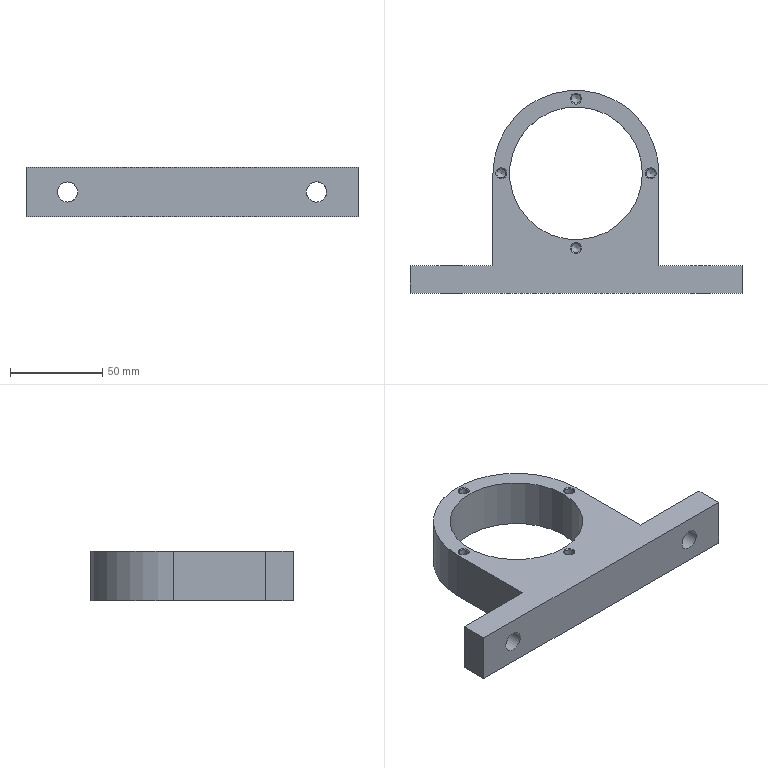Part | NX | features DATUM_CSYS 9, SKETCH 8, EXTRACT_FACE 4, HOLE PACKAGE 4, SIMPLE HOLE 4, SYMBOLIC_THREAD 4, EXTRUDE 3, Instance Feature 3, Pattern Feature 1 | 1 solid | 31 faces | box 180 x 110 x 27 mm | volume 165663 mm3 | plane 12 | cylinder 11 | cone 8 | commonest cylinder face diameters 5 x4 6 x3 11 x2 72 x1 90 x1
STEP:
#1=CARTESIAN_POINT('',(-67.5,-65.,8.));
#2=VERTEX_POINT('',#1);
#3=CARTESIAN_POINT('',(-67.5,-65.,13.5));
#4=DIRECTION('',(0.,-1.,0.));
#5=DIRECTION('',(0.,0.,-1.));
#6=AXIS2_PLACEMENT_3D('',#3,#4,#5);
#7=CIRCLE('',#6,5.5);
#8=EDGE_CURVE('',#2,#2,#7,.F.);
#9=ORIENTED_EDGE('',*,*,#8,.T.);
#10=EDGE_LOOP('',(#9));
#11=FACE_BOUND('',#10,.T.);
#12=CARTESIAN_POINT('',(67.5,-65.,8.));
#13=VERTEX_POINT('',#12);
#14=CARTESIAN_POINT('',(67.5,-65.,13.5));
#15=DIRECTION('',(0.,-1.,0.));
#16=DIRECTION('',(0.,0.,-1.));
#17=AXIS2_PLACEMENT_3D('',#14,#15,#16);
#18=CIRCLE('',#17,5.5);
#19=EDGE_CURVE('',#13,#13,#18,.T.);
#20=ORIENTED_EDGE('',*,*,#19,.F.);
#21=EDGE_LOOP('',(#20));
#22=FACE_BOUND('',#21,.T.);
#23=CARTESIAN_POINT('',(90.,-65.,0.));
#24=VERTEX_POINT('',#23);
#25=CARTESIAN_POINT('',(-90.,-65.,0.));
#26=VERTEX_POINT('',#25);
#27=CARTESIAN_POINT('',(90.,-65.,0.));
#28=DIRECTION('',(-1.,0.,0.));
#29=VECTOR('',#28,1000.);
#30=LINE('',#27,#29);
#31=EDGE_CURVE('',#24,#26,#30,.T.);
#32=ORIENTED_EDGE('',*,*,#31,.F.);
#33=CARTESIAN_POINT('',(90.,-65.,27.));
#34=VERTEX_POINT('',#33);
#35=CARTESIAN_POINT('',(90.,-65.,27.));
#36=DIRECTION('',(0.,0.,-1.));
#37=VECTOR('',#36,1000.);
#38=LINE('',#35,#37);
#39=EDGE_CURVE('',#34,#24,#38,.T.);
#40=ORIENTED_EDGE('',*,*,#39,.F.);
#41=CARTESIAN_POINT('',(-90.,-65.,27.));
#42=VERTEX_POINT('',#41);
#43=CARTESIAN_POINT('',(90.,-65.,27.));
#44=DIRECTION('',(-1.,0.,0.));
#45=VECTOR('',#44,1000.);
#46=LINE('',#43,#45);
#47=EDGE_CURVE('',#34,#42,#46,.T.);
#48=ORIENTED_EDGE('',*,*,#47,.T.);
#49=CARTESIAN_POINT('',(-90.,-65.,27.));
#50=DIRECTION('',(0.,0.,-1.));
#51=VECTOR('',#50,1000.);
#52=LINE('',#49,#51);
#53=EDGE_CURVE('',#42,#26,#52,.T.);
#54=ORIENTED_EDGE('',*,*,#53,.T.);
#55=EDGE_LOOP('',(#32,#40,#48,#54));
#56=FACE_BOUND('',#55,.T.);
#57=CARTESIAN_POINT('',(90.,-65.,27.));
#58=DIRECTION('',(0.,-1.,0.));
#59=DIRECTION('',(0.,0.,-1.));
#60=AXIS2_PLACEMENT_3D('',#57,#58,#59);
#61=PLANE('',#60);
#62=ADVANCED_FACE('',(#11,#22,#56),#61,.T.);
#63=CARTESIAN_POINT('',(-90.,-50.,0.));
#64=VERTEX_POINT('',#63);
#65=CARTESIAN_POINT('',(-90.,-65.,0.));
#66=DIRECTION('',(0.,1.,0.));
#67=VECTOR('',#66,1000.);
#68=LINE('',#65,#67);
#69=EDGE_CURVE('',#26,#64,#68,.T.);
#70=ORIENTED_EDGE('',*,*,#69,.F.);
#71=ORIENTED_EDGE('',*,*,#53,.F.);
#72=CARTESIAN_POINT('',(-90.,-50.,27.));
#73=VERTEX_POINT('',#72);
#74=CARTESIAN_POINT('',(-90.,-65.,27.));
#75=DIRECTION('',(0.,1.,0.));
#76=VECTOR('',#75,1000.);
#77=LINE('',#74,#76);
#78=EDGE_CURVE('',#42,#73,#77,.T.);
#79=ORIENTED_EDGE('',*,*,#78,.T.);
#80=CARTESIAN_POINT('',(-90.,-50.,27.));
#81=DIRECTION('',(0.,0.,-1.));
#82=VECTOR('',#81,1000.);
#83=LINE('',#80,#82);
#84=EDGE_CURVE('',#73,#64,#83,.T.);
#85=ORIENTED_EDGE('',*,*,#84,.T.);
#86=EDGE_LOOP('',(#70,#71,#79,#85));
#87=FACE_BOUND('',#86,.T.);
#88=CARTESIAN_POINT('',(-90.,-65.,27.));
#89=DIRECTION('',(-1.,0.,0.));
#90=DIRECTION('',(0.,-1.,0.));
#91=AXIS2_PLACEMENT_3D('',#88,#89,#90);
#92=PLANE('',#91);
#93=ADVANCED_FACE('',(#87),#92,.T.);
#94=CARTESIAN_POINT('',(-62.,-50.,13.5));
#95=VERTEX_POINT('',#94);
#96=CARTESIAN_POINT('',(-67.5,-50.,13.5));
#97=DIRECTION('',(0.,-1.,0.));
#98=DIRECTION('',(1.,0.,0.));
#99=AXIS2_PLACEMENT_3D('',#96,#97,#98);
#100=CIRCLE('',#99,5.5);
#101=EDGE_CURVE('',#95,#95,#100,.T.);
#102=ORIENTED_EDGE('',*,*,#101,.T.);
#103=EDGE_LOOP('',(#102));
#104=FACE_BOUND('',#103,.T.);
#105=CARTESIAN_POINT('',(-45.,-50.,0.));
#106=VERTEX_POINT('',#105);
#107=CARTESIAN_POINT('',(-90.,-50.,0.));
#108=DIRECTION('',(1.,0.,0.));
#109=VECTOR('',#108,1000.);
#110=LINE('',#107,#109);
#111=EDGE_CURVE('',#64,#106,#110,.T.);
#112=ORIENTED_EDGE('',*,*,#111,.F.);
#113=ORIENTED_EDGE('',*,*,#84,.F.);
#114=CARTESIAN_POINT('',(-45.,-50.,27.));
#115=VERTEX_POINT('',#114);
#116=CARTESIAN_POINT('',(-90.,-50.,27.));
#117=DIRECTION('',(1.,0.,0.));
#118=VECTOR('',#117,1000.);
#119=LINE('',#116,#118);
#120=EDGE_CURVE('',#73,#115,#119,.T.);
#121=ORIENTED_EDGE('',*,*,#120,.T.);
#122=CARTESIAN_POINT('',(-45.,-50.,27.));
#123=DIRECTION('',(0.,0.,-1.));
#124=VECTOR('',#123,1000.);
#125=LINE('',#122,#124);
#126=EDGE_CURVE('',#115,#106,#125,.T.);
#127=ORIENTED_EDGE('',*,*,#126,.T.);
#128=EDGE_LOOP('',(#112,#113,#121,#127));
#129=FACE_BOUND('',#128,.T.);
#130=CARTESIAN_POINT('',(-90.,-50.,27.));
#131=DIRECTION('',(0.,1.,0.));
#132=DIRECTION('',(0.,0.,1.));
#133=AXIS2_PLACEMENT_3D('',#130,#131,#132);
#134=PLANE('',#133);
#135=ADVANCED_FACE('',(#104,#129),#134,.T.);
#136=CARTESIAN_POINT('',(-45.,0.,0.));
#137=VERTEX_POINT('',#136);
#138=CARTESIAN_POINT('',(-45.,-50.,0.));
#139=DIRECTION('',(0.,1.,0.));
#140=VECTOR('',#139,1000.);
#141=LINE('',#138,#140);
#142=EDGE_CURVE('',#106,#137,#141,.T.);
#143=ORIENTED_EDGE('',*,*,#142,.F.);
#144=ORIENTED_EDGE('',*,*,#126,.F.);
#145=CARTESIAN_POINT('',(-45.,0.,27.));
#146=VERTEX_POINT('',#145);
#147=CARTESIAN_POINT('',(-45.,-50.,27.));
#148=DIRECTION('',(0.,1.,0.));
#149=VECTOR('',#148,1000.);
#150=LINE('',#147,#149);
#151=EDGE_CURVE('',#115,#146,#150,.T.);
#152=ORIENTED_EDGE('',*,*,#151,.T.);
#153=CARTESIAN_POINT('',(-45.,0.,27.));
#154=DIRECTION('',(0.,0.,-1.));
#155=VECTOR('',#154,1000.);
#156=LINE('',#153,#155);
#157=EDGE_CURVE('',#146,#137,#156,.T.);
#158=ORIENTED_EDGE('',*,*,#157,.T.);
#159=EDGE_LOOP('',(#143,#144,#152,#158));
#160=FACE_BOUND('',#159,.T.);
#161=CARTESIAN_POINT('',(-45.,-50.,27.));
#162=DIRECTION('',(-1.,0.,0.));
#163=DIRECTION('',(0.,-1.,0.));
#164=AXIS2_PLACEMENT_3D('',#161,#162,#163);
#165=PLANE('',#164);
#166=ADVANCED_FACE('',(#160),#165,.T.);
#167=CARTESIAN_POINT('',(45.,0.,0.));
#168=VERTEX_POINT('',#167);
#169=CARTESIAN_POINT('',(0.,0.,0.));
#170=DIRECTION('',(0.,0.,-1.));
#171=DIRECTION('',(1.,0.,0.));
#172=AXIS2_PLACEMENT_3D('',#169,#170,#171);
#173=CIRCLE('',#172,45.);
#174=EDGE_CURVE('',#137,#168,#173,.T.);
#175=ORIENTED_EDGE('',*,*,#174,.F.);
#176=ORIENTED_EDGE('',*,*,#157,.F.);
#177=CARTESIAN_POINT('',(45.,0.,27.));
#178=VERTEX_POINT('',#177);
#179=CARTESIAN_POINT('',(0.,0.,27.));
#180=DIRECTION('',(0.,0.,-1.));
#181=DIRECTION('',(1.,0.,0.));
#182=AXIS2_PLACEMENT_3D('',#179,#180,#181);
#183=CIRCLE('',#182,45.);
#184=EDGE_CURVE('',#146,#178,#183,.T.);
#185=ORIENTED_EDGE('',*,*,#184,.T.);
#186=CARTESIAN_POINT('',(45.,0.,27.));
#187=DIRECTION('',(0.,0.,-1.));
#188=VECTOR('',#187,1000.);
#189=LINE('',#186,#188);
#190=EDGE_CURVE('',#178,#168,#189,.T.);
#191=ORIENTED_EDGE('',*,*,#190,.T.);
#192=EDGE_LOOP('',(#175,#176,#185,#191));
#193=FACE_BOUND('',#192,.T.);
#194=CARTESIAN_POINT('',(0.,0.,27.));
#195=DIRECTION('',(0.,0.,-1.));
#196=DIRECTION('',(-1.,0.,0.));
#197=AXIS2_PLACEMENT_3D('',#194,#195,#196);
#198=CYLINDRICAL_SURFACE('',#197,45.);
#199=ADVANCED_FACE('',(#193),#198,.T.);
#200=CARTESIAN_POINT('',(45.,-50.,0.));
#201=VERTEX_POINT('',#200);
#202=CARTESIAN_POINT('',(45.,0.,0.));
#203=DIRECTION('',(0.,-1.,0.));
#204=VECTOR('',#203,1000.);
#205=LINE('',#202,#204);
#206=EDGE_CURVE('',#168,#201,#205,.T.);
#207=ORIENTED_EDGE('',*,*,#206,.F.);
#208=ORIENTED_EDGE('',*,*,#190,.F.);
#209=CARTESIAN_POINT('',(45.,-50.,27.));
#210=VERTEX_POINT('',#209);
#211=CARTESIAN_POINT('',(45.,0.,27.));
#212=DIRECTION('',(0.,-1.,0.));
#213=VECTOR('',#212,1000.);
#214=LINE('',#211,#213);
#215=EDGE_CURVE('',#178,#210,#214,.T.);
#216=ORIENTED_EDGE('',*,*,#215,.T.);
#217=CARTESIAN_POINT('',(45.,-50.,27.));
#218=DIRECTION('',(0.,0.,-1.));
#219=VECTOR('',#218,1000.);
#220=LINE('',#217,#219);
#221=EDGE_CURVE('',#210,#201,#220,.T.);
#222=ORIENTED_EDGE('',*,*,#221,.T.);
#223=EDGE_LOOP('',(#207,#208,#216,#222));
#224=FACE_BOUND('',#223,.T.);
#225=CARTESIAN_POINT('',(45.,0.,27.));
#226=DIRECTION('',(1.,0.,0.));
#227=DIRECTION('',(0.,1.,0.));
#228=AXIS2_PLACEMENT_3D('',#225,#226,#227);
#229=PLANE('',#228);
#230=ADVANCED_FACE('',(#224),#229,.T.);
#231=CARTESIAN_POINT('',(62.,-50.,13.5));
#232=VERTEX_POINT('',#231);
#233=CARTESIAN_POINT('',(67.5,-50.,13.5));
#234=DIRECTION('',(0.,1.,0.));
#235=DIRECTION('',(-1.,0.,0.));
#236=AXIS2_PLACEMENT_3D('',#233,#234,#235);
#237=CIRCLE('',#236,5.5);
#238=EDGE_CURVE('',#232,#232,#237,.T.);
#239=ORIENTED_EDGE('',*,*,#238,.F.);
#240=EDGE_LOOP('',(#239));
#241=FACE_BOUND('',#240,.T.);
#242=CARTESIAN_POINT('',(90.,-50.,0.));
#243=VERTEX_POINT('',#242);
#244=CARTESIAN_POINT('',(45.,-50.,0.));
#245=DIRECTION('',(1.,0.,0.));
#246=VECTOR('',#245,1000.);
#247=LINE('',#244,#246);
#248=EDGE_CURVE('',#201,#243,#247,.T.);
#249=ORIENTED_EDGE('',*,*,#248,.F.);
#250=ORIENTED_EDGE('',*,*,#221,.F.);
#251=CARTESIAN_POINT('',(90.,-50.,27.));
#252=VERTEX_POINT('',#251);
#253=CARTESIAN_POINT('',(45.,-50.,27.));
#254=DIRECTION('',(1.,0.,0.));
#255=VECTOR('',#254,1000.);
#256=LINE('',#253,#255);
#257=EDGE_CURVE('',#210,#252,#256,.T.);
#258=ORIENTED_EDGE('',*,*,#257,.T.);
#259=CARTESIAN_POINT('',(90.,-50.,27.));
#260=DIRECTION('',(0.,0.,-1.));
#261=VECTOR('',#260,1000.);
#262=LINE('',#259,#261);
#263=EDGE_CURVE('',#252,#243,#262,.T.);
#264=ORIENTED_EDGE('',*,*,#263,.T.);
#265=EDGE_LOOP('',(#249,#250,#258,#264));
#266=FACE_BOUND('',#265,.T.);
#267=CARTESIAN_POINT('',(45.,-50.,27.));
#268=DIRECTION('',(0.,1.,0.));
#269=DIRECTION('',(-1.,0.,0.));
#270=AXIS2_PLACEMENT_3D('',#267,#268,#269);
#271=PLANE('',#270);
#272=ADVANCED_FACE('',(#241,#266),#271,.T.);
#273=CARTESIAN_POINT('',(90.,-50.,0.));
#274=DIRECTION('',(0.,-1.,0.));
#275=VECTOR('',#274,1000.);
#276=LINE('',#273,#275);
#277=EDGE_CURVE('',#243,#24,#276,.T.);
#278=ORIENTED_EDGE('',*,*,#277,.F.);
#279=ORIENTED_EDGE('',*,*,#263,.F.);
#280=CARTESIAN_POINT('',(90.,-50.,27.));
#281=DIRECTION('',(0.,-1.,0.));
#282=VECTOR('',#281,1000.);
#283=LINE('',#280,#282);
#284=EDGE_CURVE('',#252,#34,#283,.T.);
#285=ORIENTED_EDGE('',*,*,#284,.T.);
#286=ORIENTED_EDGE('',*,*,#39,.T.);
#287=EDGE_LOOP('',(#278,#279,#285,#286));
#288=FACE_BOUND('',#287,.T.);
#289=CARTESIAN_POINT('',(90.,-50.,27.));
#290=DIRECTION('',(1.,0.,0.));
#291=DIRECTION('',(0.,1.,0.));
#292=AXIS2_PLACEMENT_3D('',#289,#290,#291);
#293=PLANE('',#292);
#294=ADVANCED_FACE('',(#288),#293,.T.);
#295=CARTESIAN_POINT('',(36.,0.,27.));
#296=VERTEX_POINT('',#295);
#297=CARTESIAN_POINT('',(0.,0.,27.));
#298=DIRECTION('',(0.,0.,-1.));
#299=DIRECTION('',(1.,0.,0.));
#300=AXIS2_PLACEMENT_3D('',#297,#298,#299);
#301=CIRCLE('',#300,36.);
#302=EDGE_CURVE('',#296,#296,#301,.T.);
#303=ORIENTED_EDGE('',*,*,#302,.F.);
#304=EDGE_LOOP('',(#303));
#305=FACE_BOUND('',#304,.T.);
#306=CARTESIAN_POINT('',(36.,0.,0.));
#307=VERTEX_POINT('',#306);
#308=CARTESIAN_POINT('',(0.,0.,0.));
#309=DIRECTION('',(0.,0.,-1.));
#310=DIRECTION('',(1.,0.,0.));
#311=AXIS2_PLACEMENT_3D('',#308,#309,#310);
#312=CIRCLE('',#311,36.);
#313=EDGE_CURVE('',#307,#307,#312,.T.);
#314=ORIENTED_EDGE('',*,*,#313,.T.);
#315=EDGE_LOOP('',(#314));
#316=FACE_BOUND('',#315,.T.);
#317=CARTESIAN_POINT('',(0.,0.,27.));
#318=DIRECTION('',(0.,0.,-1.));
#319=DIRECTION('',(-1.,0.,0.));
#320=AXIS2_PLACEMENT_3D('',#317,#318,#319);
#321=CYLINDRICAL_SURFACE('',#320,36.);
#322=ADVANCED_FACE('',(#305,#316),#321,.F.);
#323=CARTESIAN_POINT('',(-3.,40.5,27.));
#324=VERTEX_POINT('',#323);
#325=CARTESIAN_POINT('',(0.,40.5,27.));
#326=DIRECTION('',(0.,0.,-1.));
#327=DIRECTION('',(-1.,0.,0.));
#328=AXIS2_PLACEMENT_3D('',#325,#326,#327);
#329=CIRCLE('',#328,3.);
#330=EDGE_CURVE('',#324,#324,#329,.T.);
#331=ORIENTED_EDGE('',*,*,#330,.T.);
#332=EDGE_LOOP('',(#331));
#333=FACE_BOUND('',#332,.T.);
#334=CARTESIAN_POINT('',(-43.5,0.,27.));
#335=VERTEX_POINT('',#334);
#336=CARTESIAN_POINT('',(-40.5,0.,27.));
#337=DIRECTION('',(0.,0.,-1.));
#338=DIRECTION('',(-1.,0.,0.));
#339=AXIS2_PLACEMENT_3D('',#336,#337,#338);
#340=CIRCLE('',#339,3.);
#341=EDGE_CURVE('',#335,#335,#340,.T.);
#342=ORIENTED_EDGE('',*,*,#341,.T.);
#343=EDGE_LOOP('',(#342));
#344=FACE_BOUND('',#343,.T.);
#345=CARTESIAN_POINT('',(-3.,-40.5,27.));
#346=VERTEX_POINT('',#345);
#347=CARTESIAN_POINT('',(0.,-40.5,27.));
#348=DIRECTION('',(0.,0.,-1.));
#349=DIRECTION('',(-1.,0.,0.));
#350=AXIS2_PLACEMENT_3D('',#347,#348,#349);
#351=CIRCLE('',#350,3.);
#352=EDGE_CURVE('',#346,#346,#351,.T.);
#353=ORIENTED_EDGE('',*,*,#352,.T.);
#354=EDGE_LOOP('',(#353));
#355=FACE_BOUND('',#354,.T.);
#356=CARTESIAN_POINT('',(37.5,0.,27.));
#357=VERTEX_POINT('',#356);
#358=CARTESIAN_POINT('',(40.5,0.,27.));
#359=DIRECTION('',(0.,0.,-1.));
#360=DIRECTION('',(-1.,0.,0.));
#361=AXIS2_PLACEMENT_3D('',#358,#359,#360);
#362=CIRCLE('',#361,3.);
#363=EDGE_CURVE('',#357,#357,#362,.T.);
#364=ORIENTED_EDGE('',*,*,#363,.T.);
#365=EDGE_LOOP('',(#364));
#366=FACE_BOUND('',#365,.T.);
#367=ORIENTED_EDGE('',*,*,#47,.F.);
#368=ORIENTED_EDGE('',*,*,#284,.F.);
#369=ORIENTED_EDGE('',*,*,#257,.F.);
#370=ORIENTED_EDGE('',*,*,#215,.F.);
#371=ORIENTED_EDGE('',*,*,#184,.F.);
#372=ORIENTED_EDGE('',*,*,#151,.F.);
#373=ORIENTED_EDGE('',*,*,#120,.F.);
#374=ORIENTED_EDGE('',*,*,#78,.F.);
#375=EDGE_LOOP('',(#367,#368,#369,#370,#371,#372,#373,#374));
#376=FACE_BOUND('',#375,.T.);
#377=ORIENTED_EDGE('',*,*,#302,.T.);
#378=EDGE_LOOP('',(#377));
#379=FACE_BOUND('',#378,.T.);
#380=CARTESIAN_POINT('',(0.,0.,27.));
#381=DIRECTION('',(0.,0.,-1.));
#382=DIRECTION('',(-1.,0.,0.));
#383=AXIS2_PLACEMENT_3D('',#380,#381,#382);
#384=PLANE('',#383);
#385=ADVANCED_FACE('',(#333,#344,#355,#366,#376,#379),#384,.F.);
#386=CARTESIAN_POINT('',(35.708,-17.152,0.));
#387=VERTEX_POINT('',#386);
#388=CARTESIAN_POINT('',(34.208,-19.75,0.));
#389=DIRECTION('',(0.,0.,-1.));
#390=DIRECTION('',(0.5,0.866,0.));
#391=AXIS2_PLACEMENT_3D('',#388,#389,#390);
#392=CIRCLE('',#391,3.);
#393=EDGE_CURVE('',#387,#387,#392,.T.);
#394=ORIENTED_EDGE('',*,*,#393,.F.);
#395=EDGE_LOOP('',(#394));
#396=FACE_BOUND('',#395,.T.);
#397=CARTESIAN_POINT('',(-32.708,-22.348,0.));
#398=VERTEX_POINT('',#397);
#399=CARTESIAN_POINT('',(-34.208,-19.75,0.));
#400=DIRECTION('',(0.,0.,-1.));
#401=DIRECTION('',(0.5,-0.866,0.));
#402=AXIS2_PLACEMENT_3D('',#399,#400,#401);
#403=CIRCLE('',#402,3.);
#404=EDGE_CURVE('',#398,#398,#403,.T.);
#405=ORIENTED_EDGE('',*,*,#404,.F.);
#406=EDGE_LOOP('',(#405));
#407=FACE_BOUND('',#406,.T.);
#408=CARTESIAN_POINT('',(-3.,39.5,0.));
#409=VERTEX_POINT('',#408);
#410=CARTESIAN_POINT('',(0.,39.5,0.));
#411=DIRECTION('',(0.,0.,-1.));
#412=DIRECTION('',(-1.,0.,0.));
#413=AXIS2_PLACEMENT_3D('',#410,#411,#412);
#414=CIRCLE('',#413,3.);
#415=EDGE_CURVE('',#409,#409,#414,.T.);
#416=ORIENTED_EDGE('',*,*,#415,.F.);
#417=EDGE_LOOP('',(#416));
#418=FACE_BOUND('',#417,.T.);
#419=ORIENTED_EDGE('',*,*,#31,.T.);
#420=ORIENTED_EDGE('',*,*,#69,.T.);
#421=ORIENTED_EDGE('',*,*,#111,.T.);
#422=ORIENTED_EDGE('',*,*,#142,.T.);
#423=ORIENTED_EDGE('',*,*,#174,.T.);
#424=ORIENTED_EDGE('',*,*,#206,.T.);
#425=ORIENTED_EDGE('',*,*,#248,.T.);
#426=ORIENTED_EDGE('',*,*,#277,.T.);
#427=EDGE_LOOP('',(#419,#420,#421,#422,#423,#424,#425,#426));
#428=FACE_BOUND('',#427,.T.);
#429=ORIENTED_EDGE('',*,*,#313,.F.);
#430=EDGE_LOOP('',(#429));
#431=FACE_BOUND('',#430,.T.);
#432=CARTESIAN_POINT('',(0.,0.,0.));
#433=DIRECTION('',(0.,0.,-1.));
#434=DIRECTION('',(-1.,0.,0.));
#435=AXIS2_PLACEMENT_3D('',#432,#433,#434);
#436=PLANE('',#435);
#437=ADVANCED_FACE('',(#396,#407,#418,#428,#431),#436,.T.);
#438=ORIENTED_EDGE('',*,*,#19,.T.);
#439=EDGE_LOOP('',(#438));
#440=FACE_BOUND('',#439,.T.);
#441=ORIENTED_EDGE('',*,*,#238,.T.);
#442=EDGE_LOOP('',(#441));
#443=FACE_BOUND('',#442,.T.);
#444=CARTESIAN_POINT('',(67.5,-70.,13.5));
#445=DIRECTION('',(0.,1.,0.));
#446=DIRECTION('',(-1.,0.,0.));
#447=AXIS2_PLACEMENT_3D('',#444,#445,#446);
#448=CYLINDRICAL_SURFACE('',#447,5.5);
#449=ADVANCED_FACE('',(#440,#443),#448,.F.);
#450=ORIENTED_EDGE('',*,*,#8,.F.);
#451=EDGE_LOOP('',(#450));
#452=FACE_BOUND('',#451,.T.);
#453=ORIENTED_EDGE('',*,*,#101,.F.);
#454=EDGE_LOOP('',(#453));
#455=FACE_BOUND('',#454,.T.);
#456=CARTESIAN_POINT('',(-67.5,-70.,13.5));
#457=DIRECTION('',(0.,1.,0.));
#458=DIRECTION('',(-1.,0.,0.));
#459=AXIS2_PLACEMENT_3D('',#456,#457,#458);
#460=CYLINDRICAL_SURFACE('',#459,5.5);
#461=ADVANCED_FACE('',(#452,#455),#460,.F.);
#462=CARTESIAN_POINT('',(-3.,39.5,10.));
#463=VERTEX_POINT('',#462);
#464=CARTESIAN_POINT('',(0.,39.5,10.));
#465=DIRECTION('',(0.,0.,-1.));
#466=DIRECTION('',(-1.,0.,0.));
#467=AXIS2_PLACEMENT_3D('',#464,#465,#466);
#468=CIRCLE('',#467,3.);
#469=EDGE_CURVE('',#463,#463,#468,.F.);
#470=ORIENTED_EDGE('',*,*,#469,.T.);
#471=EDGE_LOOP('',(#470));
#472=FACE_BOUND('',#471,.T.);
#473=ORIENTED_EDGE('',*,*,#415,.T.);
#474=EDGE_LOOP('',(#473));
#475=FACE_BOUND('',#474,.T.);
#476=CARTESIAN_POINT('',(0.,39.5,10.));
#477=DIRECTION('',(0.,0.,-1.));
#478=DIRECTION('',(-1.,0.,0.));
#479=AXIS2_PLACEMENT_3D('',#476,#477,#478);
#480=CYLINDRICAL_SURFACE('',#479,3.);
#481=ADVANCED_FACE('',(#472,#475),#480,.F.);
#482=ORIENTED_EDGE('',*,*,#469,.F.);
#483=EDGE_LOOP('',(#482));
#484=FACE_BOUND('',#483,.T.);
#485=CARTESIAN_POINT('',(0.,39.5,10.));
#486=DIRECTION('',(0.,0.,-1.));
#487=DIRECTION('',(-1.,0.,0.));
#488=AXIS2_PLACEMENT_3D('',#485,#486,#487);
#489=PLANE('',#488);
#490=ADVANCED_FACE('',(#484),#489,.T.);
#491=CARTESIAN_POINT('',(-32.708,-22.348,10.));
#492=VERTEX_POINT('',#491);
#493=CARTESIAN_POINT('',(-34.208,-19.75,10.));
#494=DIRECTION('',(0.,0.,-1.));
#495=DIRECTION('',(0.5,-0.866,0.));
#496=AXIS2_PLACEMENT_3D('',#493,#494,#495);
#497=CIRCLE('',#496,3.);
#498=EDGE_CURVE('',#492,#492,#497,.F.);
#499=ORIENTED_EDGE('',*,*,#498,.T.);
#500=EDGE_LOOP('',(#499));
#501=FACE_BOUND('',#500,.T.);
#502=ORIENTED_EDGE('',*,*,#404,.T.);
#503=EDGE_LOOP('',(#502));
#504=FACE_BOUND('',#503,.T.);
#505=CARTESIAN_POINT('',(-34.208,-19.75,10.));
#506=DIRECTION('',(0.,0.,-1.));
#507=DIRECTION('',(-1.,0.,0.));
#508=AXIS2_PLACEMENT_3D('',#505,#506,#507);
#509=CYLINDRICAL_SURFACE('',#508,3.);
#510=ADVANCED_FACE('',(#501,#504),#509,.F.);
#511=ORIENTED_EDGE('',*,*,#498,.F.);
#512=EDGE_LOOP('',(#511));
#513=FACE_BOUND('',#512,.T.);
#514=CARTESIAN_POINT('',(-34.208,-19.75,10.));
#515=DIRECTION('',(0.,0.,-1.));
#516=DIRECTION('',(-1.,0.,0.));
#517=AXIS2_PLACEMENT_3D('',#514,#515,#516);
#518=PLANE('',#517);
#519=ADVANCED_FACE('',(#513),#518,.T.);
#520=CARTESIAN_POINT('',(35.708,-17.152,10.));
#521=VERTEX_POINT('',#520);
#522=CARTESIAN_POINT('',(34.208,-19.75,10.));
#523=DIRECTION('',(0.,0.,-1.));
#524=DIRECTION('',(0.5,0.866,0.));
#525=AXIS2_PLACEMENT_3D('',#522,#523,#524);
#526=CIRCLE('',#525,3.);
#527=EDGE_CURVE('',#521,#521,#526,.F.);
#528=ORIENTED_EDGE('',*,*,#527,.T.);
#529=EDGE_LOOP('',(#528));
#530=FACE_BOUND('',#529,.T.);
#531=ORIENTED_EDGE('',*,*,#393,.T.);
#532=EDGE_LOOP('',(#531));
#533=FACE_BOUND('',#532,.T.);
#534=CARTESIAN_POINT('',(34.208,-19.75,10.));
#535=DIRECTION('',(0.,0.,-1.));
#536=DIRECTION('',(-1.,0.,0.));
#537=AXIS2_PLACEMENT_3D('',#534,#535,#536);
#538=CYLINDRICAL_SURFACE('',#537,3.);
#539=ADVANCED_FACE('',(#530,#533),#538,.F.);
#540=ORIENTED_EDGE('',*,*,#527,.F.);
#541=EDGE_LOOP('',(#540));
#542=FACE_BOUND('',#541,.T.);
#543=CARTESIAN_POINT('',(34.208,-19.75,10.));
#544=DIRECTION('',(0.,0.,-1.));
#545=DIRECTION('',(-1.,0.,0.));
#546=AXIS2_PLACEMENT_3D('',#543,#544,#545);
#547=PLANE('',#546);
#548=ADVANCED_FACE('',(#542),#547,.T.);
#549=CARTESIAN_POINT('',(38.,0.,15.));
#550=VERTEX_POINT('',#549);
#551=CARTESIAN_POINT('',(40.5,0.,15.));
#552=DIRECTION('',(0.,0.,-1.));
#553=DIRECTION('',(-1.,0.,0.));
#554=AXIS2_PLACEMENT_3D('',#551,#552,#553);
#555=CIRCLE('',#554,2.5);
#556=EDGE_CURVE('',#550,#550,#555,.F.);
#557=ORIENTED_EDGE('',*,*,#556,.T.);
#558=EDGE_LOOP('',(#557));
#559=FACE_BOUND('',#558,.T.);
#560=CARTESIAN_POINT('',(40.5,0.,13.498));
#561=VERTEX_POINT('',#560);
#562=VERTEX_LOOP('',#561);
#563=FACE_BOUND('',#562,.T.);
#564=CARTESIAN_POINT('',(40.5,0.,15.));
#565=DIRECTION('',(0.,0.,1.));
#566=DIRECTION('',(1.,0.,0.));
#567=AXIS2_PLACEMENT_3D('',#564,#565,#566);
#568=CONICAL_SURFACE('',#567,2.5,1.03);
#569=ADVANCED_FACE('',(#559,#563),#568,.F.);
#570=CARTESIAN_POINT('',(38.,0.,26.5));
#571=VERTEX_POINT('',#570);
#572=CARTESIAN_POINT('',(40.5,0.,26.5));
#573=DIRECTION('',(0.,0.,-1.));
#574=DIRECTION('',(-1.,0.,0.));
#575=AXIS2_PLACEMENT_3D('',#572,#573,#574);
#576=CIRCLE('',#575,2.5);
#577=EDGE_CURVE('',#571,#571,#576,.F.);
#578=ORIENTED_EDGE('',*,*,#577,.T.);
#579=EDGE_LOOP('',(#578));
#580=FACE_BOUND('',#579,.T.);
#581=ORIENTED_EDGE('',*,*,#556,.F.);
#582=EDGE_LOOP('',(#581));
#583=FACE_BOUND('',#582,.T.);
#584=CARTESIAN_POINT('',(40.5,0.,27.));
#585=DIRECTION('',(0.,0.,-1.));
#586=DIRECTION('',(-1.,0.,0.));
#587=AXIS2_PLACEMENT_3D('',#584,#585,#586);
#588=CYLINDRICAL_SURFACE('',#587,2.5);
#589=ADVANCED_FACE('',(#580,#583),#588,.F.);
#590=ORIENTED_EDGE('',*,*,#577,.F.);
#591=EDGE_LOOP('',(#590));
#592=FACE_BOUND('',#591,.T.);
#593=ORIENTED_EDGE('',*,*,#363,.F.);
#594=EDGE_LOOP('',(#593));
#595=FACE_BOUND('',#594,.T.);
#596=CARTESIAN_POINT('',(40.5,0.,27.));
#597=DIRECTION('',(0.,0.,1.));
#598=DIRECTION('',(1.,0.,0.));
#599=AXIS2_PLACEMENT_3D('',#596,#597,#598);
#600=CONICAL_SURFACE('',#599,3.,0.7854);
#601=ADVANCED_FACE('',(#592,#595),#600,.F.);
#602=CARTESIAN_POINT('',(-2.5,-40.5,15.));
#603=VERTEX_POINT('',#602);
#604=CARTESIAN_POINT('',(0.,-40.5,15.));
#605=DIRECTION('',(0.,0.,-1.));
#606=DIRECTION('',(-1.,0.,0.));
#607=AXIS2_PLACEMENT_3D('',#604,#605,#606);
#608=CIRCLE('',#607,2.5);
#609=EDGE_CURVE('',#603,#603,#608,.F.);
#610=ORIENTED_EDGE('',*,*,#609,.T.);
#611=EDGE_LOOP('',(#610));
#612=FACE_BOUND('',#611,.T.);
#613=CARTESIAN_POINT('',(0.,-40.5,13.498));
#614=VERTEX_POINT('',#613);
#615=VERTEX_LOOP('',#614);
#616=FACE_BOUND('',#615,.T.);
#617=CARTESIAN_POINT('',(0.,-40.5,15.));
#618=DIRECTION('',(0.,0.,1.));
#619=DIRECTION('',(1.,0.,0.));
#620=AXIS2_PLACEMENT_3D('',#617,#618,#619);
#621=CONICAL_SURFACE('',#620,2.5,1.03);
#622=ADVANCED_FACE('',(#612,#616),#621,.F.);
#623=CARTESIAN_POINT('',(-2.5,-40.5,26.5));
#624=VERTEX_POINT('',#623);
#625=CARTESIAN_POINT('',(0.,-40.5,26.5));
#626=DIRECTION('',(0.,0.,-1.));
#627=DIRECTION('',(-1.,0.,0.));
#628=AXIS2_PLACEMENT_3D('',#625,#626,#627);
#629=CIRCLE('',#628,2.5);
#630=EDGE_CURVE('',#624,#624,#629,.F.);
#631=ORIENTED_EDGE('',*,*,#630,.T.);
#632=EDGE_LOOP('',(#631));
#633=FACE_BOUND('',#632,.T.);
#634=ORIENTED_EDGE('',*,*,#609,.F.);
#635=EDGE_LOOP('',(#634));
#636=FACE_BOUND('',#635,.T.);
#637=CARTESIAN_POINT('',(0.,-40.5,27.));
#638=DIRECTION('',(0.,0.,-1.));
#639=DIRECTION('',(-1.,0.,0.));
#640=AXIS2_PLACEMENT_3D('',#637,#638,#639);
#641=CYLINDRICAL_SURFACE('',#640,2.5);
#642=ADVANCED_FACE('',(#633,#636),#641,.F.);
#643=ORIENTED_EDGE('',*,*,#630,.F.);
#644=EDGE_LOOP('',(#643));
#645=FACE_BOUND('',#644,.T.);
#646=ORIENTED_EDGE('',*,*,#352,.F.);
#647=EDGE_LOOP('',(#646));
#648=FACE_BOUND('',#647,.T.);
#649=CARTESIAN_POINT('',(0.,-40.5,27.));
#650=DIRECTION('',(0.,0.,1.));
#651=DIRECTION('',(1.,0.,0.));
#652=AXIS2_PLACEMENT_3D('',#649,#650,#651);
#653=CONICAL_SURFACE('',#652,3.,0.7854);
#654=ADVANCED_FACE('',(#645,#648),#653,.F.);
#655=CARTESIAN_POINT('',(-43.,0.,15.));
#656=VERTEX_POINT('',#655);
#657=CARTESIAN_POINT('',(-40.5,0.,15.));
#658=DIRECTION('',(0.,0.,-1.));
#659=DIRECTION('',(-1.,0.,0.));
#660=AXIS2_PLACEMENT_3D('',#657,#658,#659);
#661=CIRCLE('',#660,2.5);
#662=EDGE_CURVE('',#656,#656,#661,.F.);
#663=ORIENTED_EDGE('',*,*,#662,.T.);
#664=EDGE_LOOP('',(#663));
#665=FACE_BOUND('',#664,.T.);
#666=CARTESIAN_POINT('',(-40.5,0.,13.498));
#667=VERTEX_POINT('',#666);
#668=VERTEX_LOOP('',#667);
#669=FACE_BOUND('',#668,.T.);
#670=CARTESIAN_POINT('',(-40.5,0.,15.));
#671=DIRECTION('',(0.,0.,1.));
#672=DIRECTION('',(1.,0.,0.));
#673=AXIS2_PLACEMENT_3D('',#670,#671,#672);
#674=CONICAL_SURFACE('',#673,2.5,1.03);
#675=ADVANCED_FACE('',(#665,#669),#674,.F.);
#676=CARTESIAN_POINT('',(-43.,0.,26.5));
#677=VERTEX_POINT('',#676);
#678=CARTESIAN_POINT('',(-40.5,0.,26.5));
#679=DIRECTION('',(0.,0.,-1.));
#680=DIRECTION('',(-1.,0.,0.));
#681=AXIS2_PLACEMENT_3D('',#678,#679,#680);
#682=CIRCLE('',#681,2.5);
#683=EDGE_CURVE('',#677,#677,#682,.F.);
#684=ORIENTED_EDGE('',*,*,#683,.T.);
#685=EDGE_LOOP('',(#684));
#686=FACE_BOUND('',#685,.T.);
#687=ORIENTED_EDGE('',*,*,#662,.F.);
#688=EDGE_LOOP('',(#687));
#689=FACE_BOUND('',#688,.T.);
#690=CARTESIAN_POINT('',(-40.5,0.,27.));
#691=DIRECTION('',(0.,0.,-1.));
#692=DIRECTION('',(-1.,0.,0.));
#693=AXIS2_PLACEMENT_3D('',#690,#691,#692);
#694=CYLINDRICAL_SURFACE('',#693,2.5);
#695=ADVANCED_FACE('',(#686,#689),#694,.F.);
#696=ORIENTED_EDGE('',*,*,#683,.F.);
#697=EDGE_LOOP('',(#696));
#698=FACE_BOUND('',#697,.T.);
#699=ORIENTED_EDGE('',*,*,#341,.F.);
#700=EDGE_LOOP('',(#699));
#701=FACE_BOUND('',#700,.T.);
#702=CARTESIAN_POINT('',(-40.5,0.,27.));
#703=DIRECTION('',(0.,0.,1.));
#704=DIRECTION('',(1.,0.,0.));
#705=AXIS2_PLACEMENT_3D('',#702,#703,#704);
#706=CONICAL_SURFACE('',#705,3.,0.7854);
#707=ADVANCED_FACE('',(#698,#701),#706,.F.);
#708=CARTESIAN_POINT('',(-2.5,40.5,15.));
#709=VERTEX_POINT('',#708);
#710=CARTESIAN_POINT('',(0.,40.5,15.));
#711=DIRECTION('',(0.,0.,-1.));
#712=DIRECTION('',(-1.,0.,0.));
#713=AXIS2_PLACEMENT_3D('',#710,#711,#712);
#714=CIRCLE('',#713,2.5);
#715=EDGE_CURVE('',#709,#709,#714,.F.);
#716=ORIENTED_EDGE('',*,*,#715,.T.);
#717=EDGE_LOOP('',(#716));
#718=FACE_BOUND('',#717,.T.);
#719=CARTESIAN_POINT('',(0.,40.5,13.498));
#720=VERTEX_POINT('',#719);
#721=VERTEX_LOOP('',#720);
#722=FACE_BOUND('',#721,.T.);
#723=CARTESIAN_POINT('',(0.,40.5,15.));
#724=DIRECTION('',(0.,0.,1.));
#725=DIRECTION('',(1.,0.,0.));
#726=AXIS2_PLACEMENT_3D('',#723,#724,#725);
#727=CONICAL_SURFACE('',#726,2.5,1.03);
#728=ADVANCED_FACE('',(#718,#722),#727,.F.);
#729=CARTESIAN_POINT('',(-2.5,40.5,26.5));
#730=VERTEX_POINT('',#729);
#731=CARTESIAN_POINT('',(0.,40.5,26.5));
#732=DIRECTION('',(0.,0.,-1.));
#733=DIRECTION('',(-1.,0.,0.));
#734=AXIS2_PLACEMENT_3D('',#731,#732,#733);
#735=CIRCLE('',#734,2.5);
#736=EDGE_CURVE('',#730,#730,#735,.F.);
#737=ORIENTED_EDGE('',*,*,#736,.T.);
#738=EDGE_LOOP('',(#737));
#739=FACE_BOUND('',#738,.T.);
#740=ORIENTED_EDGE('',*,*,#715,.F.);
#741=EDGE_LOOP('',(#740));
#742=FACE_BOUND('',#741,.T.);
#743=CARTESIAN_POINT('',(0.,40.5,27.));
#744=DIRECTION('',(0.,0.,-1.));
#745=DIRECTION('',(-1.,0.,0.));
#746=AXIS2_PLACEMENT_3D('',#743,#744,#745);
#747=CYLINDRICAL_SURFACE('',#746,2.5);
#748=ADVANCED_FACE('',(#739,#742),#747,.F.);
#749=ORIENTED_EDGE('',*,*,#736,.F.);
#750=EDGE_LOOP('',(#749));
#751=FACE_BOUND('',#750,.T.);
#752=ORIENTED_EDGE('',*,*,#330,.F.);
#753=EDGE_LOOP('',(#752));
#754=FACE_BOUND('',#753,.T.);
#755=CARTESIAN_POINT('',(0.,40.5,27.));
#756=DIRECTION('',(0.,0.,1.));
#757=DIRECTION('',(1.,0.,0.));
#758=AXIS2_PLACEMENT_3D('',#755,#756,#757);
#759=CONICAL_SURFACE('',#758,3.,0.7854);
#760=ADVANCED_FACE('',(#751,#754),#759,.F.);
#761=CLOSED_SHELL('',(#62,#93,#135,#166,#199,#230,#272,#294,#322,#385,#437,#449,#461,#481,#490,#510,#519,#539,#548,#569,#589,#601,#622,#642,#654,#675,#695,#707,#728,#748,#760));
#762=MANIFOLD_SOLID_BREP('',#761);
#763=(LENGTH_UNIT()NAMED_UNIT(*)SI_UNIT(.MILLI.,.METRE.));
#764=UNCERTAINTY_MEASURE_WITH_UNIT(LENGTH_MEASURE(0.00001),#763,'','');
#765=(NAMED_UNIT(*)PLANE_ANGLE_UNIT()SI_UNIT($,.RADIAN.));
#766=(NAMED_UNIT(*)SI_UNIT($,.STERADIAN.)SOLID_ANGLE_UNIT());
#767=(GEOMETRIC_REPRESENTATION_CONTEXT(3)GLOBAL_UNCERTAINTY_ASSIGNED_CONTEXT((#764))GLOBAL_UNIT_ASSIGNED_CONTEXT((#763,#765,#766))REPRESENTATION_CONTEXT('',''));
#768=ADVANCED_BREP_SHAPE_REPRESENTATION('',(#762),#767);